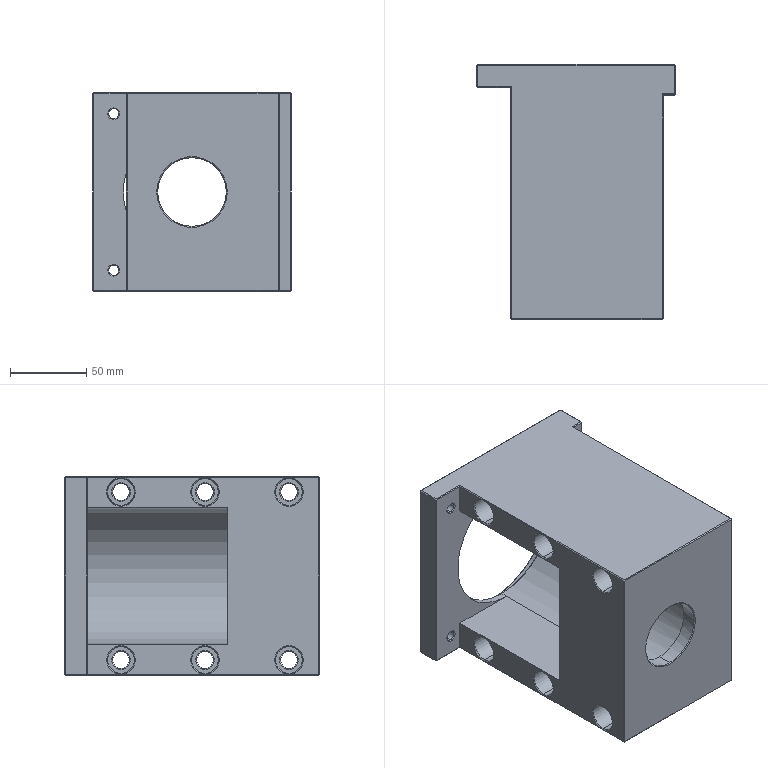Part | SolidWorks | features BaseBody 1 | 1 solid | 167 faces | box 130 x 167 x 130 mm | volume 1161837 mm3 | cone 64 | plane 59 | cylinder 44 | commonest cylinder face diameters 11 x12 17.5 x12 6.5 x8 12 x4 45 x2 62 x2